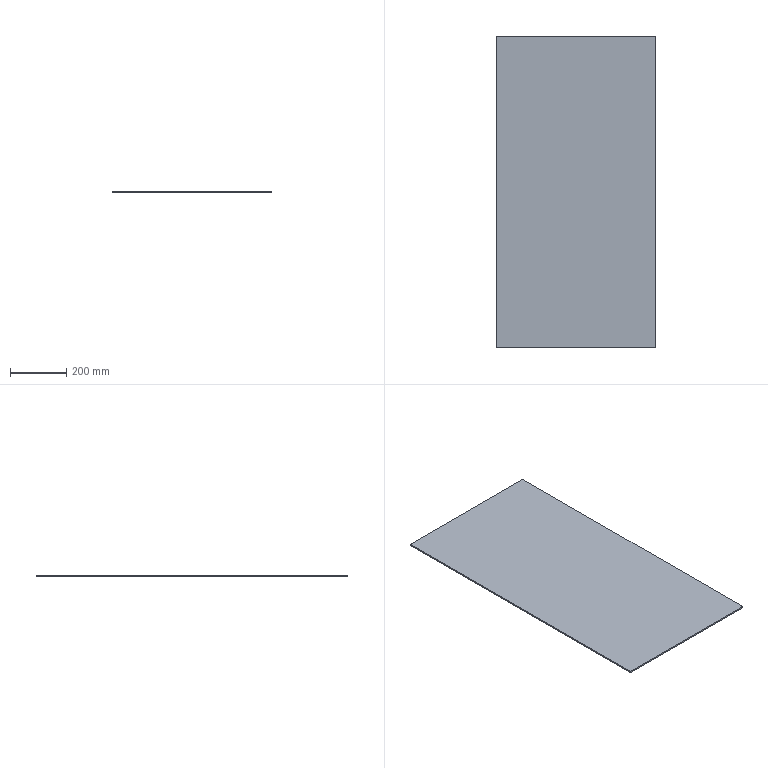Part | SolidWorks | features Fillet 1, FlatPattern 1, SMBaseFlange 1, SheetMetal 1 | 1 solid | 7 faces | box 565 x 1106 x 5 mm | volume 3122985 mm3 | plane 6 | cylinder 1 | commonest cylinder face diameters 14 x1
STEP:
#1=CARTESIAN_POINT('',(282.5,-545.75,5.));
#2=VERTEX_POINT('',#1);
#3=CARTESIAN_POINT('',(282.5,552.75,5.));
#4=VERTEX_POINT('',#3);
#5=CARTESIAN_POINT('',(282.5,552.75,5.));
#6=DIRECTION('',(0.,1.,0.));
#7=VECTOR('',#6,1000.);
#8=LINE('',#5,#7);
#9=EDGE_CURVE('',#2,#4,#8,.T.);
#10=ORIENTED_EDGE('',*,*,#9,.F.);
#11=CARTESIAN_POINT('',(282.5,-545.75,0.));
#12=VERTEX_POINT('',#11);
#13=CARTESIAN_POINT('',(282.5,-545.75,5.));
#14=DIRECTION('',(0.,0.,-1.));
#15=VECTOR('',#14,1000.);
#16=LINE('',#13,#15);
#17=EDGE_CURVE('',#2,#12,#16,.T.);
#18=ORIENTED_EDGE('',*,*,#17,.T.);
#19=CARTESIAN_POINT('',(282.5,552.75,0.));
#20=VERTEX_POINT('',#19);
#21=CARTESIAN_POINT('',(282.5,552.75,0.));
#22=DIRECTION('',(0.,1.,0.));
#23=VECTOR('',#22,1000.);
#24=LINE('',#21,#23);
#25=EDGE_CURVE('',#12,#20,#24,.T.);
#26=ORIENTED_EDGE('',*,*,#25,.T.);
#27=CARTESIAN_POINT('',(282.5,552.75,5.));
#28=DIRECTION('',(0.,0.,-1.));
#29=VECTOR('',#28,1000.);
#30=LINE('',#27,#29);
#31=EDGE_CURVE('',#4,#20,#30,.T.);
#32=ORIENTED_EDGE('',*,*,#31,.F.);
#33=EDGE_LOOP('',(#10,#18,#26,#32));
#34=FACE_OUTER_BOUND('',#33,.T.);
#35=CARTESIAN_POINT('',(282.5,552.75,5.));
#36=DIRECTION('',(-1.,0.,0.));
#37=DIRECTION('',(0.,-1.,0.));
#38=AXIS2_PLACEMENT_3D('',#35,#36,#37);
#39=PLANE('',#38);
#40=ADVANCED_FACE('',(#34),#39,.F.);
#41=CARTESIAN_POINT('',(-282.5,552.75,0.));
#42=VERTEX_POINT('',#41);
#43=CARTESIAN_POINT('',(-282.5,552.75,0.));
#44=DIRECTION('',(-1.,0.,0.));
#45=VECTOR('',#44,1000.);
#46=LINE('',#43,#45);
#47=EDGE_CURVE('',#20,#42,#46,.T.);
#48=ORIENTED_EDGE('',*,*,#47,.T.);
#49=CARTESIAN_POINT('',(-282.5,552.75,5.));
#50=VERTEX_POINT('',#49);
#51=CARTESIAN_POINT('',(-282.5,552.75,5.));
#52=DIRECTION('',(0.,0.,-1.));
#53=VECTOR('',#52,1000.);
#54=LINE('',#51,#53);
#55=EDGE_CURVE('',#50,#42,#54,.T.);
#56=ORIENTED_EDGE('',*,*,#55,.F.);
#57=CARTESIAN_POINT('',(-282.5,552.75,5.));
#58=DIRECTION('',(-1.,0.,0.));
#59=VECTOR('',#58,1000.);
#60=LINE('',#57,#59);
#61=EDGE_CURVE('',#4,#50,#60,.T.);
#62=ORIENTED_EDGE('',*,*,#61,.F.);
#63=ORIENTED_EDGE('',*,*,#31,.T.);
#64=EDGE_LOOP('',(#48,#56,#62,#63));
#65=FACE_OUTER_BOUND('',#64,.T.);
#66=CARTESIAN_POINT('',(-282.5,552.75,5.));
#67=DIRECTION('',(0.,-1.,0.));
#68=DIRECTION('',(0.,0.,-1.));
#69=AXIS2_PLACEMENT_3D('',#66,#67,#68);
#70=PLANE('',#69);
#71=ADVANCED_FACE('',(#65),#70,.F.);
#72=CARTESIAN_POINT('',(-282.5,-552.75,0.));
#73=VERTEX_POINT('',#72);
#74=CARTESIAN_POINT('',(-282.5,552.75,0.));
#75=DIRECTION('',(0.,-1.,0.));
#76=VECTOR('',#75,1000.);
#77=LINE('',#74,#76);
#78=EDGE_CURVE('',#42,#73,#77,.T.);
#79=ORIENTED_EDGE('',*,*,#78,.T.);
#80=CARTESIAN_POINT('',(-282.5,-552.75,5.));
#81=VERTEX_POINT('',#80);
#82=CARTESIAN_POINT('',(-282.5,-552.75,5.));
#83=DIRECTION('',(0.,0.,-1.));
#84=VECTOR('',#83,1000.);
#85=LINE('',#82,#84);
#86=EDGE_CURVE('',#81,#73,#85,.T.);
#87=ORIENTED_EDGE('',*,*,#86,.F.);
#88=CARTESIAN_POINT('',(-282.5,552.75,5.));
#89=DIRECTION('',(0.,-1.,0.));
#90=VECTOR('',#89,1000.);
#91=LINE('',#88,#90);
#92=EDGE_CURVE('',#50,#81,#91,.T.);
#93=ORIENTED_EDGE('',*,*,#92,.F.);
#94=ORIENTED_EDGE('',*,*,#55,.T.);
#95=EDGE_LOOP('',(#79,#87,#93,#94));
#96=FACE_OUTER_BOUND('',#95,.T.);
#97=CARTESIAN_POINT('',(-282.5,552.75,5.));
#98=DIRECTION('',(1.,0.,0.));
#99=DIRECTION('',(0.,1.,0.));
#100=AXIS2_PLACEMENT_3D('',#97,#98,#99);
#101=PLANE('',#100);
#102=ADVANCED_FACE('',(#96),#101,.F.);
#103=CARTESIAN_POINT('',(275.5,-552.75,0.));
#104=VERTEX_POINT('',#103);
#105=CARTESIAN_POINT('',(-282.5,-552.75,0.));
#106=DIRECTION('',(1.,0.,0.));
#107=VECTOR('',#106,1000.);
#108=LINE('',#105,#107);
#109=EDGE_CURVE('',#73,#104,#108,.T.);
#110=ORIENTED_EDGE('',*,*,#109,.T.);
#111=CARTESIAN_POINT('',(275.5,-552.75,5.));
#112=VERTEX_POINT('',#111);
#113=CARTESIAN_POINT('',(275.5,-552.75,5.));
#114=DIRECTION('',(0.,0.,1.));
#115=VECTOR('',#114,1000.);
#116=LINE('',#113,#115);
#117=EDGE_CURVE('',#104,#112,#116,.T.);
#118=ORIENTED_EDGE('',*,*,#117,.T.);
#119=CARTESIAN_POINT('',(-282.5,-552.75,5.));
#120=DIRECTION('',(1.,0.,0.));
#121=VECTOR('',#120,1000.);
#122=LINE('',#119,#121);
#123=EDGE_CURVE('',#81,#112,#122,.T.);
#124=ORIENTED_EDGE('',*,*,#123,.F.);
#125=ORIENTED_EDGE('',*,*,#86,.T.);
#126=EDGE_LOOP('',(#110,#118,#124,#125));
#127=FACE_OUTER_BOUND('',#126,.T.);
#128=CARTESIAN_POINT('',(-282.5,-552.75,5.));
#129=DIRECTION('',(0.,1.,0.));
#130=DIRECTION('',(0.,0.,1.));
#131=AXIS2_PLACEMENT_3D('',#128,#129,#130);
#132=PLANE('',#131);
#133=ADVANCED_FACE('',(#127),#132,.F.);
#134=ORIENTED_EDGE('',*,*,#123,.T.);
#135=CARTESIAN_POINT('',(275.5,-545.75,5.));
#136=DIRECTION('',(0.,0.,1.));
#137=DIRECTION('',(1.,0.,0.));
#138=AXIS2_PLACEMENT_3D('',#135,#136,#137);
#139=CIRCLE('',#138,7.);
#140=EDGE_CURVE('',#112,#2,#139,.T.);
#141=ORIENTED_EDGE('',*,*,#140,.T.);
#142=ORIENTED_EDGE('',*,*,#9,.T.);
#143=ORIENTED_EDGE('',*,*,#61,.T.);
#144=ORIENTED_EDGE('',*,*,#92,.T.);
#145=EDGE_LOOP('',(#134,#141,#142,#143,#144));
#146=FACE_OUTER_BOUND('',#145,.T.);
#147=CARTESIAN_POINT('',(0.,0.,5.));
#148=DIRECTION('',(0.,0.,1.));
#149=DIRECTION('',(1.,0.,0.));
#150=AXIS2_PLACEMENT_3D('',#147,#148,#149);
#151=PLANE('',#150);
#152=ADVANCED_FACE('',(#146),#151,.T.);
#153=ORIENTED_EDGE('',*,*,#25,.F.);
#154=CARTESIAN_POINT('',(275.5,-545.75,0.));
#155=DIRECTION('',(0.,0.,-1.));
#156=DIRECTION('',(1.,0.,0.));
#157=AXIS2_PLACEMENT_3D('',#154,#155,#156);
#158=CIRCLE('',#157,7.);
#159=EDGE_CURVE('',#12,#104,#158,.T.);
#160=ORIENTED_EDGE('',*,*,#159,.T.);
#161=ORIENTED_EDGE('',*,*,#109,.F.);
#162=ORIENTED_EDGE('',*,*,#78,.F.);
#163=ORIENTED_EDGE('',*,*,#47,.F.);
#164=EDGE_LOOP('',(#153,#160,#161,#162,#163));
#165=FACE_OUTER_BOUND('',#164,.T.);
#166=CARTESIAN_POINT('',(0.,0.,0.));
#167=DIRECTION('',(0.,0.,1.));
#168=DIRECTION('',(1.,0.,0.));
#169=AXIS2_PLACEMENT_3D('',#166,#167,#168);
#170=PLANE('',#169);
#171=ADVANCED_FACE('',(#165),#170,.F.);
#172=ORIENTED_EDGE('',*,*,#140,.F.);
#173=ORIENTED_EDGE('',*,*,#117,.F.);
#174=ORIENTED_EDGE('',*,*,#159,.F.);
#175=ORIENTED_EDGE('',*,*,#17,.F.);
#176=EDGE_LOOP('',(#172,#173,#174,#175));
#177=FACE_OUTER_BOUND('',#176,.T.);
#178=CARTESIAN_POINT('',(275.5,-545.75,5.));
#179=DIRECTION('',(0.,0.,-1.));
#180=DIRECTION('',(-1.,0.,0.));
#181=AXIS2_PLACEMENT_3D('',#178,#179,#180);
#182=CYLINDRICAL_SURFACE('',#181,7.);
#183=ADVANCED_FACE('',(#177),#182,.T.);
#184=CLOSED_SHELL('',(#40,#71,#102,#133,#152,#171,#183));
#185=MANIFOLD_SOLID_BREP('',#184);
#186=CARTESIAN_POINT('',(0.,0.,0.));
#187=DIRECTION('',(0.,0.,1.));
#188=DIRECTION('',(1.,0.,0.));
#189=AXIS2_PLACEMENT_3D('',#186,#187,#188);
#190=(LENGTH_UNIT()NAMED_UNIT(*)SI_UNIT(.MILLI.,.METRE.));
#191=UNCERTAINTY_MEASURE_WITH_UNIT(LENGTH_MEASURE(0.00001),#190,'','');
#192=(NAMED_UNIT(*)PLANE_ANGLE_UNIT()SI_UNIT($,.RADIAN.));
#193=(NAMED_UNIT(*)SI_UNIT($,.STERADIAN.)SOLID_ANGLE_UNIT());
#194=(GEOMETRIC_REPRESENTATION_CONTEXT(3)GLOBAL_UNCERTAINTY_ASSIGNED_CONTEXT((#191))GLOBAL_UNIT_ASSIGNED_CONTEXT((#190,#192,#193))REPRESENTATION_CONTEXT('',''));
#195=ADVANCED_BREP_SHAPE_REPRESENTATION('',(#185,#189),#194);